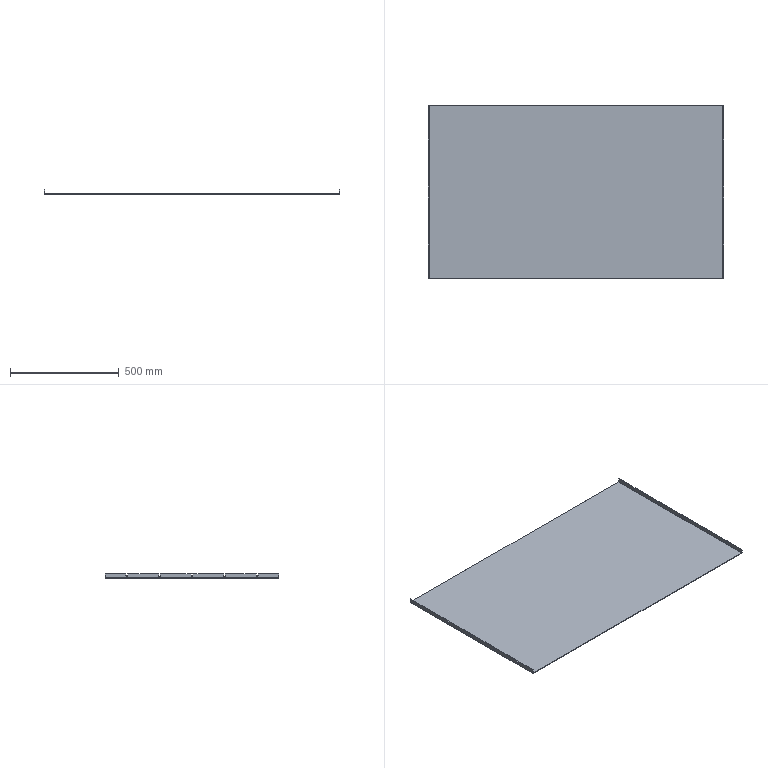Part | SolidWorks | features EdgeFlange 1, FlatPattern 1, ICE 1, LPattern 1, MirrorPattern 1, SMBaseFlange 1, SheetMetal 1 | 1 solid | 67 faces | box 1360 x 800 x 20 mm | volume 3338438 mm3 | plane 48 | cylinder 19 | commonest cylinder face diameters 8 x15 1.473 x2 7.473 x2